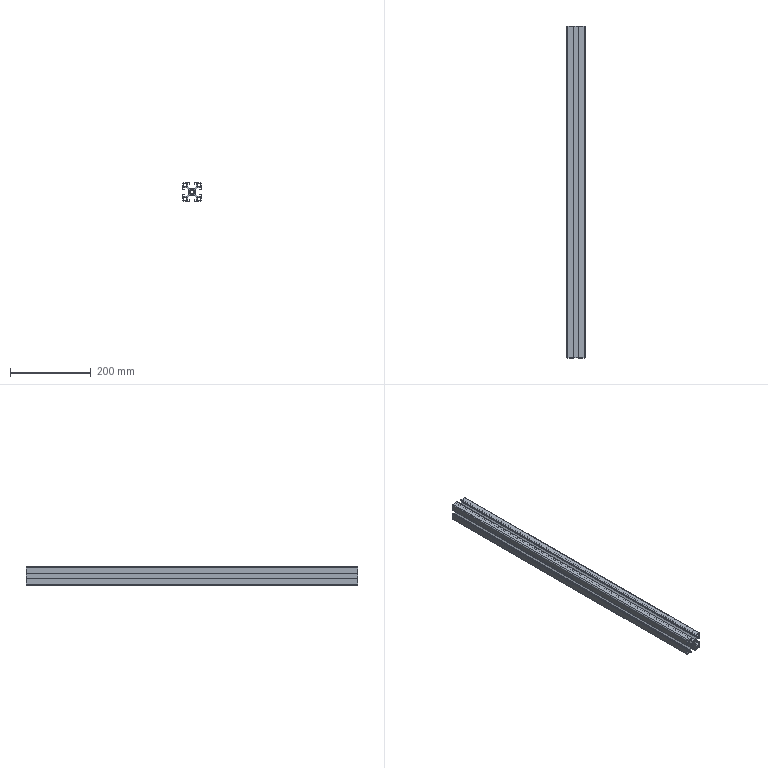Part | STEP file | 1 solid | 135 faces | box 45 x 820 x 45 mm | volume 567678 mm3 | plane 118 | cylinder 17 | commonest cylinder face diameters 10 x9 3 x4 5 x4